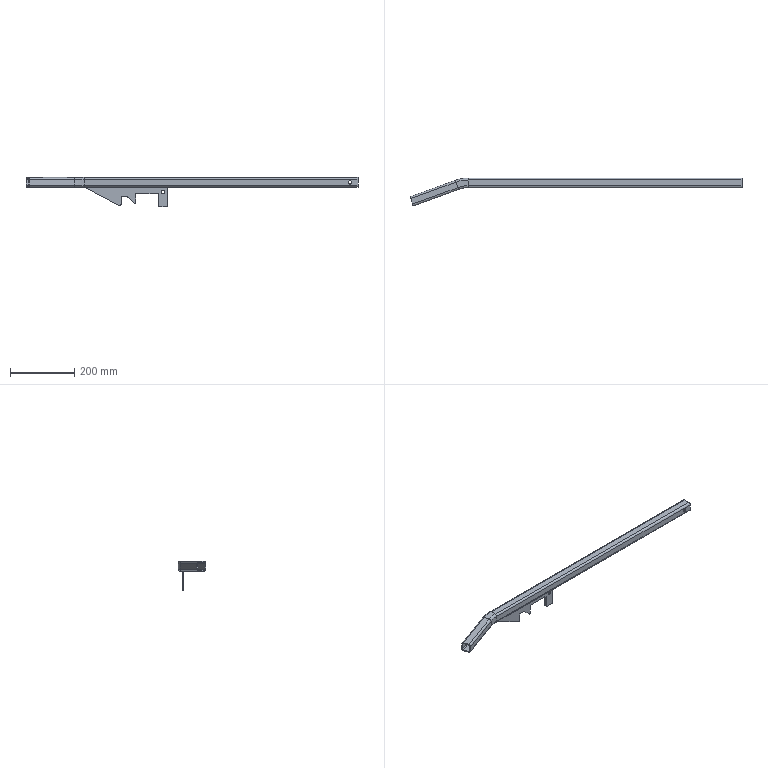Part | SolidWorks | features HoleWzd 2, ICE 1, WeldMemberFeat 1, WeldmentFeature 1 | 4 solids | 79 faces | box 1030 x 86.429 x 90 mm | volume 351764 mm3 | plane 38 | cylinder 33 | torus 8 | commonest cylinder face diameters 6 x8 12 x8 10 x7 11 x4 4 x2 170 x1